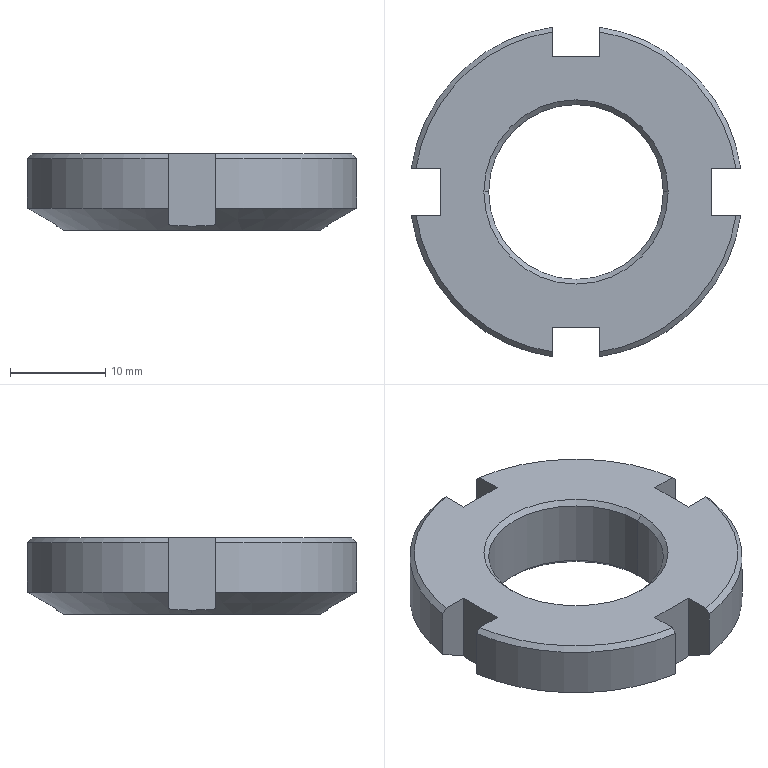Part | STEP file | PN_0042_Default<As Machined> | 1 solid | 30 faces | box 34.641 x 34.641 x 8 mm | volume 4654 mm3 | plane 14 | cone 10 | cylinder 6 | commonest cylinder face diameters 35 x4 18.376 x2
STEP:
#1=CARTESIAN_POINT('',(-9.188,0.,7.5));
#2=VERTEX_POINT('',#1);
#3=CARTESIAN_POINT('',(9.188,0.,7.5));
#4=VERTEX_POINT('',#3);
#5=CARTESIAN_POINT('',(0.,0.,7.5));
#6=DIRECTION('',(0.,0.,1.));
#7=AXIS2_PLACEMENT_3D('',#5,#6,$);
#8=CIRCLE('',#7,9.188);
#9=EDGE_CURVE('',#2,#4,#8,.T.);
#10=ORIENTED_EDGE('',*,*,#9,.F.);
#11=CARTESIAN_POINT('',(-9.688,0.,8.));
#12=VERTEX_POINT('',#11);
#13=CARTESIAN_POINT('',(-353557.985,0.,353556.297));
#14=DIRECTION('',(-0.7071,0.,0.7071));
#15=VECTOR('',#14,1.);
#16=LINE('',#13,#15);
#17=EDGE_CURVE('',#2,#12,#16,.T.);
#18=ORIENTED_EDGE('',*,*,#17,.T.);
#19=CARTESIAN_POINT('',(9.688,0.,8.));
#20=VERTEX_POINT('',#19);
#21=CARTESIAN_POINT('',(0.,0.,8.));
#22=DIRECTION('',(0.,0.,1.));
#23=AXIS2_PLACEMENT_3D('',#21,#22,$);
#24=CIRCLE('',#23,9.688);
#25=EDGE_CURVE('',#20,#12,#24,.F.);
#26=ORIENTED_EDGE('',*,*,#25,.F.);
#27=CARTESIAN_POINT('',(353557.985,0.,353556.297));
#28=DIRECTION('',(0.7071,0.,0.7071));
#29=VECTOR('',#28,1.);
#30=LINE('',#27,#29);
#31=EDGE_CURVE('',#4,#20,#30,.T.);
#32=ORIENTED_EDGE('',*,*,#31,.F.);
#33=EDGE_LOOP('',(#10,#18,#26,#32));
#34=FACE_OUTER_BOUND('',#33,.T.);
#35=CARTESIAN_POINT('',(0.,0.,7.5));
#36=DIRECTION('',(0.,0.,1.));
#37=DIRECTION('',(-1.,0.,0.));
#38=AXIS2_PLACEMENT_3D('',#35,#36,#37);
#39=CONICAL_SURFACE('',#38,9.188,0.7854);
#40=ADVANCED_FACE('',(#34),#39,.F.);
#41=ORIENTED_EDGE('',*,*,#9,.T.);
#42=CARTESIAN_POINT('',(9.188,0.,0.5));
#43=VERTEX_POINT('',#42);
#44=CARTESIAN_POINT('',(9.188,0.,8.));
#45=DIRECTION('',(0.,0.,-1.));
#46=VECTOR('',#45,1.);
#47=LINE('',#44,#46);
#48=EDGE_CURVE('',#4,#43,#47,.T.);
#49=ORIENTED_EDGE('',*,*,#48,.T.);
#50=CARTESIAN_POINT('',(-9.188,0.,0.5));
#51=VERTEX_POINT('',#50);
#52=CARTESIAN_POINT('',(0.,0.,0.5));
#53=DIRECTION('',(0.,0.,-1.));
#54=AXIS2_PLACEMENT_3D('',#52,#53,$);
#55=CIRCLE('',#54,9.188);
#56=EDGE_CURVE('',#43,#51,#55,.T.);
#57=ORIENTED_EDGE('',*,*,#56,.T.);
#58=CARTESIAN_POINT('',(-9.188,0.,8.));
#59=DIRECTION('',(0.,0.,-1.));
#60=VECTOR('',#59,1.);
#61=LINE('',#58,#60);
#62=EDGE_CURVE('',#2,#51,#61,.T.);
#63=ORIENTED_EDGE('',*,*,#62,.F.);
#64=EDGE_LOOP('',(#41,#49,#57,#63));
#65=FACE_OUTER_BOUND('',#64,.T.);
#66=CARTESIAN_POINT('',(0.,0.,8.));
#67=DIRECTION('',(0.,0.,-1.));
#68=DIRECTION('',(1.,0.,0.));
#69=AXIS2_PLACEMENT_3D('',#66,#67,#68);
#70=CYLINDRICAL_SURFACE('',#69,9.188);
#71=ADVANCED_FACE('',(#65),#70,.F.);
#72=ORIENTED_EDGE('',*,*,#17,.F.);
#73=CARTESIAN_POINT('',(0.,0.,7.5));
#74=DIRECTION('',(0.,0.,1.));
#75=AXIS2_PLACEMENT_3D('',#73,#74,$);
#76=CIRCLE('',#75,9.188);
#77=EDGE_CURVE('',#4,#2,#76,.T.);
#78=ORIENTED_EDGE('',*,*,#77,.F.);
#79=ORIENTED_EDGE('',*,*,#31,.T.);
#80=CARTESIAN_POINT('',(0.,0.,8.));
#81=DIRECTION('',(0.,0.,1.));
#82=AXIS2_PLACEMENT_3D('',#80,#81,$);
#83=CIRCLE('',#82,9.688);
#84=EDGE_CURVE('',#12,#20,#83,.F.);
#85=ORIENTED_EDGE('',*,*,#84,.F.);
#86=EDGE_LOOP('',(#72,#78,#79,#85));
#87=FACE_OUTER_BOUND('',#86,.T.);
#88=CARTESIAN_POINT('',(0.,0.,7.5));
#89=DIRECTION('',(0.,0.,1.));
#90=DIRECTION('',(1.,0.,0.));
#91=AXIS2_PLACEMENT_3D('',#88,#89,#90);
#92=CONICAL_SURFACE('',#91,9.188,0.7854);
#93=ADVANCED_FACE('',(#87),#92,.F.);
#94=CARTESIAN_POINT('',(16.815,2.5,8.));
#95=VERTEX_POINT('',#94);
#96=CARTESIAN_POINT('',(14.221,2.5,8.));
#97=VERTEX_POINT('',#96);
#98=CARTESIAN_POINT('',(15.518,2.5,8.));
#99=DIRECTION('',(-1.,0.,0.));
#100=VECTOR('',#99,1.);
#101=LINE('',#98,#100);
#102=EDGE_CURVE('',#95,#97,#101,.T.);
#103=ORIENTED_EDGE('',*,*,#102,.F.);
#104=CARTESIAN_POINT('',(2.5,16.815,8.));
#105=VERTEX_POINT('',#104);
#106=CARTESIAN_POINT('',(-0.000000003,-0.000000003,8.));
#107=DIRECTION('',(0.,0.,1.));
#108=AXIS2_PLACEMENT_3D('',#106,#107,$);
#109=CIRCLE('',#108,17.);
#110=EDGE_CURVE('',#95,#105,#109,.T.);
#111=ORIENTED_EDGE('',*,*,#110,.T.);
#112=CARTESIAN_POINT('',(2.5,14.221,8.));
#113=VERTEX_POINT('',#112);
#114=CARTESIAN_POINT('',(2.5,15.518,8.));
#115=DIRECTION('',(0.,1.,0.));
#116=VECTOR('',#115,1.);
#117=LINE('',#114,#116);
#118=EDGE_CURVE('',#113,#105,#117,.T.);
#119=ORIENTED_EDGE('',*,*,#118,.F.);
#120=CARTESIAN_POINT('',(-2.5,14.221,8.));
#121=VERTEX_POINT('',#120);
#122=CARTESIAN_POINT('',(0.,14.221,8.));
#123=DIRECTION('',(1.,0.,0.));
#124=VECTOR('',#123,1.);
#125=LINE('',#122,#124);
#126=EDGE_CURVE('',#121,#113,#125,.T.);
#127=ORIENTED_EDGE('',*,*,#126,.F.);
#128=CARTESIAN_POINT('',(-2.5,16.815,8.));
#129=VERTEX_POINT('',#128);
#130=CARTESIAN_POINT('',(-2.5,15.518,8.));
#131=DIRECTION('',(0.,-1.,0.));
#132=VECTOR('',#131,1.);
#133=LINE('',#130,#132);
#134=EDGE_CURVE('',#129,#121,#133,.T.);
#135=ORIENTED_EDGE('',*,*,#134,.F.);
#136=CARTESIAN_POINT('',(-16.815,2.5,8.));
#137=VERTEX_POINT('',#136);
#138=CARTESIAN_POINT('',(0.000000003,-0.000000003,8.));
#139=DIRECTION('',(0.,0.,1.));
#140=AXIS2_PLACEMENT_3D('',#138,#139,$);
#141=CIRCLE('',#140,17.);
#142=EDGE_CURVE('',#129,#137,#141,.T.);
#143=ORIENTED_EDGE('',*,*,#142,.T.);
#144=CARTESIAN_POINT('',(-14.221,2.5,8.));
#145=VERTEX_POINT('',#144);
#146=CARTESIAN_POINT('',(-15.518,2.5,8.));
#147=DIRECTION('',(-1.,0.,0.));
#148=VECTOR('',#147,1.);
#149=LINE('',#146,#148);
#150=EDGE_CURVE('',#145,#137,#149,.T.);
#151=ORIENTED_EDGE('',*,*,#150,.F.);
#152=CARTESIAN_POINT('',(-14.221,-2.5,8.));
#153=VERTEX_POINT('',#152);
#154=CARTESIAN_POINT('',(-14.221,0.,8.));
#155=DIRECTION('',(0.,1.,0.));
#156=VECTOR('',#155,1.);
#157=LINE('',#154,#156);
#158=EDGE_CURVE('',#153,#145,#157,.T.);
#159=ORIENTED_EDGE('',*,*,#158,.F.);
#160=CARTESIAN_POINT('',(-16.815,-2.5,8.));
#161=VERTEX_POINT('',#160);
#162=CARTESIAN_POINT('',(-15.518,-2.5,8.));
#163=DIRECTION('',(1.,0.,0.));
#164=VECTOR('',#163,1.);
#165=LINE('',#162,#164);
#166=EDGE_CURVE('',#161,#153,#165,.T.);
#167=ORIENTED_EDGE('',*,*,#166,.F.);
#168=CARTESIAN_POINT('',(-2.5,-16.815,8.));
#169=VERTEX_POINT('',#168);
#170=CARTESIAN_POINT('',(0.000000003,0.000000003,8.));
#171=DIRECTION('',(0.,0.,1.));
#172=AXIS2_PLACEMENT_3D('',#170,#171,$);
#173=CIRCLE('',#172,17.);
#174=EDGE_CURVE('',#161,#169,#173,.T.);
#175=ORIENTED_EDGE('',*,*,#174,.T.);
#176=CARTESIAN_POINT('',(-2.5,-14.221,8.));
#177=VERTEX_POINT('',#176);
#178=CARTESIAN_POINT('',(-2.5,-15.518,8.));
#179=DIRECTION('',(0.,-1.,0.));
#180=VECTOR('',#179,1.);
#181=LINE('',#178,#180);
#182=EDGE_CURVE('',#177,#169,#181,.T.);
#183=ORIENTED_EDGE('',*,*,#182,.F.);
#184=CARTESIAN_POINT('',(2.5,-14.221,8.));
#185=VERTEX_POINT('',#184);
#186=CARTESIAN_POINT('',(0.,-14.221,8.));
#187=DIRECTION('',(-1.,0.,0.));
#188=VECTOR('',#187,1.);
#189=LINE('',#186,#188);
#190=EDGE_CURVE('',#185,#177,#189,.T.);
#191=ORIENTED_EDGE('',*,*,#190,.F.);
#192=CARTESIAN_POINT('',(2.5,-16.815,8.));
#193=VERTEX_POINT('',#192);
#194=CARTESIAN_POINT('',(2.5,-15.518,8.));
#195=DIRECTION('',(0.,1.,0.));
#196=VECTOR('',#195,1.);
#197=LINE('',#194,#196);
#198=EDGE_CURVE('',#193,#185,#197,.T.);
#199=ORIENTED_EDGE('',*,*,#198,.F.);
#200=CARTESIAN_POINT('',(16.815,-2.5,8.));
#201=VERTEX_POINT('',#200);
#202=CARTESIAN_POINT('',(-0.000000003,0.000000003,8.));
#203=DIRECTION('',(0.,0.,1.));
#204=AXIS2_PLACEMENT_3D('',#202,#203,$);
#205=CIRCLE('',#204,17.);
#206=EDGE_CURVE('',#193,#201,#205,.T.);
#207=ORIENTED_EDGE('',*,*,#206,.T.);
#208=CARTESIAN_POINT('',(14.221,-2.5,8.));
#209=VERTEX_POINT('',#208);
#210=CARTESIAN_POINT('',(15.518,-2.5,8.));
#211=DIRECTION('',(1.,0.,0.));
#212=VECTOR('',#211,1.);
#213=LINE('',#210,#212);
#214=EDGE_CURVE('',#209,#201,#213,.T.);
#215=ORIENTED_EDGE('',*,*,#214,.F.);
#216=CARTESIAN_POINT('',(14.221,0.,8.));
#217=DIRECTION('',(0.,-1.,0.));
#218=VECTOR('',#217,1.);
#219=LINE('',#216,#218);
#220=EDGE_CURVE('',#97,#209,#219,.T.);
#221=ORIENTED_EDGE('',*,*,#220,.F.);
#222=EDGE_LOOP('',(#103,#111,#119,#127,#135,#143,#151,#159,#167,#175,#183,#191,#199,#207,#215,#221));
#223=FACE_OUTER_BOUND('',#222,.T.);
#224=ORIENTED_EDGE('',*,*,#25,.T.);
#225=ORIENTED_EDGE('',*,*,#84,.T.);
#226=EDGE_LOOP('',(#224,#225));
#227=FACE_BOUND('',#226,.T.);
#228=CARTESIAN_POINT('',(0.,0.,8.));
#229=DIRECTION('',(0.,0.,1.));
#230=DIRECTION('',(1.,0.,0.));
#231=AXIS2_PLACEMENT_3D('',#228,#229,#230);
#232=PLANE('',#231);
#233=ADVANCED_FACE('',(#223,#227),#232,.T.);
#234=ORIENTED_EDGE('',*,*,#48,.F.);
#235=ORIENTED_EDGE('',*,*,#77,.T.);
#236=ORIENTED_EDGE('',*,*,#62,.T.);
#237=CARTESIAN_POINT('',(0.,0.,0.5));
#238=DIRECTION('',(0.,0.,-1.));
#239=AXIS2_PLACEMENT_3D('',#237,#238,$);
#240=CIRCLE('',#239,9.188);
#241=EDGE_CURVE('',#51,#43,#240,.T.);
#242=ORIENTED_EDGE('',*,*,#241,.T.);
#243=EDGE_LOOP('',(#234,#235,#236,#242));
#244=FACE_OUTER_BOUND('',#243,.T.);
#245=CARTESIAN_POINT('',(0.,0.,8.));
#246=DIRECTION('',(0.,0.,-1.));
#247=DIRECTION('',(-1.,0.,0.));
#248=AXIS2_PLACEMENT_3D('',#245,#246,#247);
#249=CYLINDRICAL_SURFACE('',#248,9.188);
#250=ADVANCED_FACE('',(#244),#249,.F.);
#251=ORIENTED_EDGE('',*,*,#56,.F.);
#252=CARTESIAN_POINT('',(9.688,0.,0.));
#253=VERTEX_POINT('',#252);
#254=CARTESIAN_POINT('',(353558.235,0.,-353548.547));
#255=DIRECTION('',(0.7071,0.,-0.7071));
#256=VECTOR('',#255,1.);
#257=LINE('',#254,#256);
#258=EDGE_CURVE('',#43,#253,#257,.T.);
#259=ORIENTED_EDGE('',*,*,#258,.T.);
#260=CARTESIAN_POINT('',(-9.688,0.,0.));
#261=VERTEX_POINT('',#260);
#262=CARTESIAN_POINT('',(0.,0.,0.));
#263=DIRECTION('',(0.,0.,-1.));
#264=AXIS2_PLACEMENT_3D('',#262,#263,$);
#265=CIRCLE('',#264,9.688);
#266=EDGE_CURVE('',#261,#253,#265,.F.);
#267=ORIENTED_EDGE('',*,*,#266,.F.);
#268=CARTESIAN_POINT('',(-353558.235,0.,-353548.547));
#269=DIRECTION('',(-0.7071,0.,-0.7071));
#270=VECTOR('',#269,1.);
#271=LINE('',#268,#270);
#272=EDGE_CURVE('',#51,#261,#271,.T.);
#273=ORIENTED_EDGE('',*,*,#272,.F.);
#274=EDGE_LOOP('',(#251,#259,#267,#273));
#275=FACE_OUTER_BOUND('',#274,.T.);
#276=CARTESIAN_POINT('',(0.,0.,0.));
#277=DIRECTION('',(0.,0.,-1.));
#278=DIRECTION('',(1.,0.,0.));
#279=AXIS2_PLACEMENT_3D('',#276,#277,#278);
#280=CONICAL_SURFACE('',#279,9.688,0.7854);
#281=ADVANCED_FACE('',(#275),#280,.F.);
#282=CARTESIAN_POINT('',(17.321,2.5,7.5));
#283=VERTEX_POINT('',#282);
#284=CARTESIAN_POINT('',(17.321,2.5,7.5));
#285=CARTESIAN_POINT('',(17.219,2.5,7.6));
#286=CARTESIAN_POINT('',(17.118,2.5,7.7));
#287=CARTESIAN_POINT('',(17.017,2.5,7.8));
#288=CARTESIAN_POINT('',(16.916,2.5,7.9));
#289=CARTESIAN_POINT('',(16.815,2.5,8.));
#290=B_SPLINE_CURVE_WITH_KNOTS('',5,(#284,#285,#286,#287,#288,#289),.UNSPECIFIED.,.F.,.U.,(6,6),(0.,1.005),.UNSPECIFIED.);
#291=EDGE_CURVE('',#283,#95,#290,.T.);
#292=ORIENTED_EDGE('',*,*,#291,.T.);
#293=ORIENTED_EDGE('',*,*,#102,.T.);
#294=CARTESIAN_POINT('',(14.221,2.5,0.5419));
#295=VERTEX_POINT('',#294);
#296=CARTESIAN_POINT('',(14.221,2.5,4.271));
#297=DIRECTION('',(0.,0.,1.));
#298=VECTOR('',#297,1.);
#299=LINE('',#296,#298);
#300=EDGE_CURVE('',#295,#97,#299,.T.);
#301=ORIENTED_EDGE('',*,*,#300,.F.);
#302=CARTESIAN_POINT('',(17.321,2.5,2.309));
#303=VERTEX_POINT('',#302);
#304=CARTESIAN_POINT('',(14.221,2.5,0.5419));
#305=CARTESIAN_POINT('',(14.841,2.5,0.8947));
#306=CARTESIAN_POINT('',(15.461,2.5,1.248));
#307=CARTESIAN_POINT('',(16.081,2.5,1.601));
#308=CARTESIAN_POINT('',(16.701,2.5,1.955));
#309=CARTESIAN_POINT('',(17.321,2.5,2.309));
#310=B_SPLINE_CURVE_WITH_KNOTS('',5,(#304,#305,#306,#307,#308,#309),.UNSPECIFIED.,.F.,.U.,(6,6),(0.,5.047),.UNSPECIFIED.);
#311=EDGE_CURVE('',#295,#303,#310,.T.);
#312=ORIENTED_EDGE('',*,*,#311,.T.);
#313=CARTESIAN_POINT('',(17.321,2.5,4.905));
#314=DIRECTION('',(0.,0.,1.));
#315=VECTOR('',#314,1.);
#316=LINE('',#313,#315);
#317=EDGE_CURVE('',#303,#283,#316,.T.);
#318=ORIENTED_EDGE('',*,*,#317,.T.);
#319=EDGE_LOOP('',(#292,#293,#301,#312,#318));
#320=FACE_OUTER_BOUND('',#319,.T.);
#321=CARTESIAN_POINT('',(14.221,2.5,0.));
#322=DIRECTION('',(0.,1.,0.));
#323=DIRECTION('',(-1.,0.,0.));
#324=AXIS2_PLACEMENT_3D('',#321,#322,#323);
#325=PLANE('',#324);
#326=ADVANCED_FACE('',(#320),#325,.F.);
#327=ORIENTED_EDGE('',*,*,#291,.F.);
#328=CARTESIAN_POINT('',(2.5,17.321,7.5));
#329=VERTEX_POINT('',#328);
#330=CARTESIAN_POINT('',(0.,0.,7.5));
#331=DIRECTION('',(0.,0.,-1.));
#332=AXIS2_PLACEMENT_3D('',#330,#331,$);
#333=CIRCLE('',#332,17.5);
#334=EDGE_CURVE('',#329,#283,#333,.T.);
#335=ORIENTED_EDGE('',*,*,#334,.F.);
#336=CARTESIAN_POINT('',(2.5,16.815,8.));
#337=CARTESIAN_POINT('',(2.5,16.983,7.834));
#338=CARTESIAN_POINT('',(2.5,17.151,7.667));
#339=CARTESIAN_POINT('',(2.5,17.321,7.5));
#340=B_SPLINE_CURVE_WITH_KNOTS('',3,(#336,#337,#338,#339),.UNSPECIFIED.,.F.,.U.,(4,4),(0.,1.089),.UNSPECIFIED.);
#341=EDGE_CURVE('',#105,#329,#340,.T.);
#342=ORIENTED_EDGE('',*,*,#341,.F.);
#343=ORIENTED_EDGE('',*,*,#110,.F.);
#344=EDGE_LOOP('',(#327,#335,#342,#343));
#345=FACE_OUTER_BOUND('',#344,.T.);
#346=CARTESIAN_POINT('',(0.,0.,8.));
#347=DIRECTION('',(0.,0.,-1.));
#348=DIRECTION('',(-1.,0.,0.));
#349=AXIS2_PLACEMENT_3D('',#346,#347,#348);
#350=CONICAL_SURFACE('',#349,17.,0.7854);
#351=ADVANCED_FACE('',(#345),#350,.T.);
#352=ORIENTED_EDGE('',*,*,#341,.T.);
#353=CARTESIAN_POINT('',(2.5,17.321,2.309));
#354=VERTEX_POINT('',#353);
#355=CARTESIAN_POINT('',(2.5,17.321,4.905));
#356=DIRECTION('',(0.,0.,1.));
#357=VECTOR('',#356,1.);
#358=LINE('',#355,#357);
#359=EDGE_CURVE('',#354,#329,#358,.T.);
#360=ORIENTED_EDGE('',*,*,#359,.F.);
#361=CARTESIAN_POINT('',(2.5,14.221,0.5419));
#362=VERTEX_POINT('',#361);
#363=CARTESIAN_POINT('',(2.5,17.321,2.309));
#364=CARTESIAN_POINT('',(2.5,16.701,1.955));
#365=CARTESIAN_POINT('',(2.5,16.081,1.601));
#366=CARTESIAN_POINT('',(2.5,15.461,1.248));
#367=CARTESIAN_POINT('',(2.5,14.841,0.8947));
#368=CARTESIAN_POINT('',(2.5,14.221,0.5419));
#369=B_SPLINE_CURVE_WITH_KNOTS('',5,(#363,#364,#365,#366,#367,#368),.UNSPECIFIED.,.F.,.U.,(6,6),(0.,5.047),.UNSPECIFIED.);
#370=EDGE_CURVE('',#354,#362,#369,.T.);
#371=ORIENTED_EDGE('',*,*,#370,.T.);
#372=CARTESIAN_POINT('',(2.5,14.221,4.271));
#373=DIRECTION('',(0.,0.,1.));
#374=VECTOR('',#373,1.);
#375=LINE('',#372,#374);
#376=EDGE_CURVE('',#362,#113,#375,.T.);
#377=ORIENTED_EDGE('',*,*,#376,.T.);
#378=ORIENTED_EDGE('',*,*,#118,.T.);
#379=EDGE_LOOP('',(#352,#360,#371,#377,#378));
#380=FACE_OUTER_BOUND('',#379,.T.);
#381=CARTESIAN_POINT('',(2.5,14.221,0.));
#382=DIRECTION('',(1.,0.,0.));
#383=DIRECTION('',(0.,1.,0.));
#384=AXIS2_PLACEMENT_3D('',#381,#382,#383);
#385=PLANE('',#384);
#386=ADVANCED_FACE('',(#380),#385,.F.);
#387=CARTESIAN_POINT('',(-2.5,14.221,0.5419));
#388=VERTEX_POINT('',#387);
#389=CARTESIAN_POINT('',(2.5,14.221,0.5419));
#390=CARTESIAN_POINT('',(1.904,14.221,0.4823));
#391=CARTESIAN_POINT('',(1.307,14.221,0.44));
#392=CARTESIAN_POINT('',(0.7073,14.221,0.4152));
#393=CARTESIAN_POINT('',(-0.2936,14.221,0.4047));
#394=CARTESIAN_POINT('',(-1.296,14.221,0.4451));
#395=CARTESIAN_POINT('',(-1.697,14.221,0.4695));
#396=CARTESIAN_POINT('',(-2.099,14.221,0.5018));
#397=CARTESIAN_POINT('',(-2.5,14.221,0.5419));
#398=B_SPLINE_CURVE_WITH_KNOTS('',5,(#389,#390,#391,#392,#393,#394,#395,#396,#397),.UNSPECIFIED.,.F.,.U.,(6,3,6),(0.,4.243,7.085),.UNSPECIFIED.);
#399=EDGE_CURVE('',#362,#388,#398,.T.);
#400=ORIENTED_EDGE('',*,*,#399,.T.);
#401=CARTESIAN_POINT('',(-2.5,14.221,4.271));
#402=DIRECTION('',(0.,0.,1.));
#403=VECTOR('',#402,1.);
#404=LINE('',#401,#403);
#405=EDGE_CURVE('',#388,#121,#404,.T.);
#406=ORIENTED_EDGE('',*,*,#405,.T.);
#407=ORIENTED_EDGE('',*,*,#126,.T.);
#408=ORIENTED_EDGE('',*,*,#376,.F.);
#409=EDGE_LOOP('',(#400,#406,#407,#408));
#410=FACE_OUTER_BOUND('',#409,.T.);
#411=CARTESIAN_POINT('',(2.5,14.221,0.));
#412=DIRECTION('',(0.,-1.,0.));
#413=DIRECTION('',(1.,0.,0.));
#414=AXIS2_PLACEMENT_3D('',#411,#412,#413);
#415=PLANE('',#414);
#416=ADVANCED_FACE('',(#410),#415,.F.);
#417=CARTESIAN_POINT('',(-2.5,17.321,7.5));
#418=VERTEX_POINT('',#417);
#419=CARTESIAN_POINT('',(-2.5,17.321,7.5));
#420=CARTESIAN_POINT('',(-2.5,17.219,7.6));
#421=CARTESIAN_POINT('',(-2.5,17.118,7.7));
#422=CARTESIAN_POINT('',(-2.5,17.017,7.8));
#423=CARTESIAN_POINT('',(-2.5,16.916,7.9));
#424=CARTESIAN_POINT('',(-2.5,16.815,8.));
#425=B_SPLINE_CURVE_WITH_KNOTS('',5,(#419,#420,#421,#422,#423,#424),.UNSPECIFIED.,.F.,.U.,(6,6),(0.,1.005),.UNSPECIFIED.);
#426=EDGE_CURVE('',#418,#129,#425,.T.);
#427=ORIENTED_EDGE('',*,*,#426,.T.);
#428=ORIENTED_EDGE('',*,*,#134,.T.);
#429=ORIENTED_EDGE('',*,*,#405,.F.);
#430=CARTESIAN_POINT('',(-2.5,17.321,2.309));
#431=VERTEX_POINT('',#430);
#432=CARTESIAN_POINT('',(-2.5,14.221,0.5419));
#433=CARTESIAN_POINT('',(-2.5,14.841,0.8947));
#434=CARTESIAN_POINT('',(-2.5,15.461,1.248));
#435=CARTESIAN_POINT('',(-2.5,16.081,1.601));
#436=CARTESIAN_POINT('',(-2.5,16.701,1.955));
#437=CARTESIAN_POINT('',(-2.5,17.321,2.309));
#438=B_SPLINE_CURVE_WITH_KNOTS('',5,(#432,#433,#434,#435,#436,#437),.UNSPECIFIED.,.F.,.U.,(6,6),(0.,5.047),.UNSPECIFIED.);
#439=EDGE_CURVE('',#388,#431,#438,.T.);
#440=ORIENTED_EDGE('',*,*,#439,.T.);
#441=CARTESIAN_POINT('',(-2.5,17.321,4.905));
#442=DIRECTION('',(0.,0.,1.));
#443=VECTOR('',#442,1.);
#444=LINE('',#441,#443);
#445=EDGE_CURVE('',#431,#418,#444,.T.);
#446=ORIENTED_EDGE('',*,*,#445,.T.);
#447=EDGE_LOOP('',(#427,#428,#429,#440,#446));
#448=FACE_OUTER_BOUND('',#447,.T.);
#449=CARTESIAN_POINT('',(-2.5,14.221,0.));
#450=DIRECTION('',(-1.,0.,0.));
#451=DIRECTION('',(0.,-1.,0.));
#452=AXIS2_PLACEMENT_3D('',#449,#450,#451);
#453=PLANE('',#452);
#454=ADVANCED_FACE('',(#448),#453,.F.);
#455=ORIENTED_EDGE('',*,*,#426,.F.);
#456=CARTESIAN_POINT('',(-17.321,2.5,7.5));
#457=VERTEX_POINT('',#456);
#458=CARTESIAN_POINT('',(0.,0.,7.5));
#459=DIRECTION('',(0.,0.,-1.));
#460=AXIS2_PLACEMENT_3D('',#458,#459,$);
#461=CIRCLE('',#460,17.5);
#462=EDGE_CURVE('',#457,#418,#461,.T.);
#463=ORIENTED_EDGE('',*,*,#462,.F.);
#464=CARTESIAN_POINT('',(-16.815,2.5,8.));
#465=CARTESIAN_POINT('',(-16.983,2.5,7.834));
#466=CARTESIAN_POINT('',(-17.151,2.5,7.667));
#467=CARTESIAN_POINT('',(-17.321,2.5,7.5));
#468=B_SPLINE_CURVE_WITH_KNOTS('',3,(#464,#465,#466,#467),.UNSPECIFIED.,.F.,.U.,(4,4),(0.,1.089),.UNSPECIFIED.);
#469=EDGE_CURVE('',#137,#457,#468,.T.);
#470=ORIENTED_EDGE('',*,*,#469,.F.);
#471=ORIENTED_EDGE('',*,*,#142,.F.);
#472=EDGE_LOOP('',(#455,#463,#470,#471));
#473=FACE_OUTER_BOUND('',#472,.T.);
#474=CARTESIAN_POINT('',(0.,0.,8.));
#475=DIRECTION('',(0.,0.,-1.));
#476=DIRECTION('',(-1.,0.,0.));
#477=AXIS2_PLACEMENT_3D('',#474,#475,#476);
#478=CONICAL_SURFACE('',#477,17.,0.7854);
#479=ADVANCED_FACE('',(#473),#478,.T.);
#480=ORIENTED_EDGE('',*,*,#469,.T.);
#481=CARTESIAN_POINT('',(-17.321,2.5,2.309));
#482=VERTEX_POINT('',#481);
#483=CARTESIAN_POINT('',(-17.321,2.5,4.905));
#484=DIRECTION('',(0.,0.,1.));
#485=VECTOR('',#484,1.);
#486=LINE('',#483,#485);
#487=EDGE_CURVE('',#482,#457,#486,.T.);
#488=ORIENTED_EDGE('',*,*,#487,.F.);
#489=CARTESIAN_POINT('',(-14.221,2.5,0.5419));
#490=VERTEX_POINT('',#489);
#491=CARTESIAN_POINT('',(-17.321,2.5,2.309));
#492=CARTESIAN_POINT('',(-16.701,2.5,1.955));
#493=CARTESIAN_POINT('',(-16.081,2.5,1.601));
#494=CARTESIAN_POINT('',(-15.461,2.5,1.248));
#495=CARTESIAN_POINT('',(-14.841,2.5,0.8947));
#496=CARTESIAN_POINT('',(-14.221,2.5,0.5419));
#497=B_SPLINE_CURVE_WITH_KNOTS('',5,(#491,#492,#493,#494,#495,#496),.UNSPECIFIED.,.F.,.U.,(6,6),(0.,5.047),.UNSPECIFIED.);
#498=EDGE_CURVE('',#482,#490,#497,.T.);
#499=ORIENTED_EDGE('',*,*,#498,.T.);
#500=CARTESIAN_POINT('',(-14.221,2.5,4.271));
#501=DIRECTION('',(0.,0.,1.));
#502=VECTOR('',#501,1.);
#503=LINE('',#500,#502);
#504=EDGE_CURVE('',#490,#145,#503,.T.);
#505=ORIENTED_EDGE('',*,*,#504,.T.);
#506=ORIENTED_EDGE('',*,*,#150,.T.);
#507=EDGE_LOOP('',(#480,#488,#499,#505,#506));
#508=FACE_OUTER_BOUND('',#507,.T.);
#509=CARTESIAN_POINT('',(-14.221,2.5,0.));
#510=DIRECTION('',(0.,1.,0.));
#511=DIRECTION('',(-1.,0.,0.));
#512=AXIS2_PLACEMENT_3D('',#509,#510,#511);
#513=PLANE('',#512);
#514=ADVANCED_FACE('',(#508),#513,.F.);
#515=CARTESIAN_POINT('',(-14.221,0.,0.416));
#516=VERTEX_POINT('',#515);
#517=CARTESIAN_POINT('',(-14.221,2.5,0.5419));
#518=CARTESIAN_POINT('',(-14.221,2.002,0.4921));
#519=CARTESIAN_POINT('',(-14.221,1.503,0.4543));
#520=CARTESIAN_POINT('',(-14.221,1.002,0.4288));
#521=CARTESIAN_POINT('',(-14.221,0.5013,0.416));
#522=CARTESIAN_POINT('',(-14.221,0.,0.416));
#523=B_SPLINE_CURVE_WITH_KNOTS('',5,(#517,#518,#519,#520,#521,#522),.UNSPECIFIED.,.F.,.U.,(6,6),(0.,3.541),.UNSPECIFIED.);
#524=EDGE_CURVE('',#490,#516,#523,.T.);
#525=ORIENTED_EDGE('',*,*,#524,.T.);
#526=CARTESIAN_POINT('',(-14.221,-2.5,0.5419));
#527=VERTEX_POINT('',#526);
#528=CARTESIAN_POINT('',(-14.221,0.,0.416));
#529=CARTESIAN_POINT('',(-14.221,-0.2993,0.416));
#530=CARTESIAN_POINT('',(-14.221,-0.5986,0.4205));
#531=CARTESIAN_POINT('',(-14.221,-0.8998,0.4297));
#532=CARTESIAN_POINT('',(-14.221,-1.4,0.4525));
#533=CARTESIAN_POINT('',(-14.221,-1.9,0.4878));
#534=CARTESIAN_POINT('',(-14.221,-2.1,0.5039));
#535=CARTESIAN_POINT('',(-14.221,-2.3,0.5219));
#536=CARTESIAN_POINT('',(-14.221,-2.5,0.5419));
#537=B_SPLINE_CURVE_WITH_KNOTS('',5,(#528,#529,#530,#531,#532,#533,#534,#535,#536),.UNSPECIFIED.,.F.,.U.,(6,3,6),(0.,2.121,3.539),.UNSPECIFIED.);
#538=EDGE_CURVE('',#516,#527,#537,.T.);
#539=ORIENTED_EDGE('',*,*,#538,.T.);
#540=CARTESIAN_POINT('',(-14.221,-2.5,4.271));
#541=DIRECTION('',(0.,0.,1.));
#542=VECTOR('',#541,1.);
#543=LINE('',#540,#542);
#544=EDGE_CURVE('',#527,#153,#543,.T.);
#545=ORIENTED_EDGE('',*,*,#544,.T.);
#546=ORIENTED_EDGE('',*,*,#158,.T.);
#547=ORIENTED_EDGE('',*,*,#504,.F.);
#548=EDGE_LOOP('',(#525,#539,#545,#546,#547));
#549=FACE_OUTER_BOUND('',#548,.T.);
#550=CARTESIAN_POINT('',(-14.221,2.5,0.));
#551=DIRECTION('',(1.,0.,0.));
#552=DIRECTION('',(0.,1.,0.));
#553=AXIS2_PLACEMENT_3D('',#550,#551,#552);
#554=PLANE('',#553);
#555=ADVANCED_FACE('',(#549),#554,.F.);
#556=CARTESIAN_POINT('',(-17.321,-2.5,7.5));
#557=VERTEX_POINT('',#556);
#558=CARTESIAN_POINT('',(-17.321,-2.5,7.5));
#559=CARTESIAN_POINT('',(-17.219,-2.5,7.6));
#560=CARTESIAN_POINT('',(-17.118,-2.5,7.7));
#561=CARTESIAN_POINT('',(-17.017,-2.5,7.8));
#562=CARTESIAN_POINT('',(-16.916,-2.5,7.9));
#563=CARTESIAN_POINT('',(-16.815,-2.5,8.));
#564=B_SPLINE_CURVE_WITH_KNOTS('',5,(#558,#559,#560,#561,#562,#563),.UNSPECIFIED.,.F.,.U.,(6,6),(0.,1.005),.UNSPECIFIED.);
#565=EDGE_CURVE('',#557,#161,#564,.T.);
#566=ORIENTED_EDGE('',*,*,#565,.T.);
#567=ORIENTED_EDGE('',*,*,#166,.T.);
#568=ORIENTED_EDGE('',*,*,#544,.F.);
#569=CARTESIAN_POINT('',(-17.321,-2.5,2.309));
#570=VERTEX_POINT('',#569);
#571=CARTESIAN_POINT('',(-14.221,-2.5,0.5419));
#572=CARTESIAN_POINT('',(-14.841,-2.5,0.8947));
#573=CARTESIAN_POINT('',(-15.461,-2.5,1.248));
#574=CARTESIAN_POINT('',(-16.081,-2.5,1.601));
#575=CARTESIAN_POINT('',(-16.701,-2.5,1.955));
#576=CARTESIAN_POINT('',(-17.321,-2.5,2.309));
#577=B_SPLINE_CURVE_WITH_KNOTS('',5,(#571,#572,#573,#574,#575,#576),.UNSPECIFIED.,.F.,.U.,(6,6),(0.,5.047),.UNSPECIFIED.);
#578=EDGE_CURVE('',#527,#570,#577,.T.);
#579=ORIENTED_EDGE('',*,*,#578,.T.);
#580=CARTESIAN_POINT('',(-17.321,-2.5,4.905));
#581=DIRECTION('',(0.,0.,1.));
#582=VECTOR('',#581,1.);
#583=LINE('',#580,#582);
#584=EDGE_CURVE('',#570,#557,#583,.T.);
#585=ORIENTED_EDGE('',*,*,#584,.T.);
#586=EDGE_LOOP('',(#566,#567,#568,#579,#585));
#587=FACE_OUTER_BOUND('',#586,.T.);
#588=CARTESIAN_POINT('',(-14.221,-2.5,0.));
#589=DIRECTION('',(0.,-1.,0.));
#590=DIRECTION('',(1.,0.,0.));
#591=AXIS2_PLACEMENT_3D('',#588,#589,#590);
#592=PLANE('',#591);
#593=ADVANCED_FACE('',(#587),#592,.F.);
#594=ORIENTED_EDGE('',*,*,#565,.F.);
#595=CARTESIAN_POINT('',(-2.5,-17.321,7.5));
#596=VERTEX_POINT('',#595);
#597=CARTESIAN_POINT('',(0.,0.,7.5));
#598=DIRECTION('',(0.,0.,-1.));
#599=AXIS2_PLACEMENT_3D('',#597,#598,$);
#600=CIRCLE('',#599,17.5);
#601=EDGE_CURVE('',#596,#557,#600,.T.);
#602=ORIENTED_EDGE('',*,*,#601,.F.);
#603=CARTESIAN_POINT('',(-2.5,-16.815,8.));
#604=CARTESIAN_POINT('',(-2.5,-16.983,7.834));
#605=CARTESIAN_POINT('',(-2.5,-17.151,7.667));
#606=CARTESIAN_POINT('',(-2.5,-17.321,7.5));
#607=B_SPLINE_CURVE_WITH_KNOTS('',3,(#603,#604,#605,#606),.UNSPECIFIED.,.F.,.U.,(4,4),(0.,1.089),.UNSPECIFIED.);
#608=EDGE_CURVE('',#169,#596,#607,.T.);
#609=ORIENTED_EDGE('',*,*,#608,.F.);
#610=ORIENTED_EDGE('',*,*,#174,.F.);
#611=EDGE_LOOP('',(#594,#602,#609,#610));
#612=FACE_OUTER_BOUND('',#611,.T.);
#613=CARTESIAN_POINT('',(0.,0.,8.));
#614=DIRECTION('',(0.,0.,-1.));
#615=DIRECTION('',(1.,0.,0.));
#616=AXIS2_PLACEMENT_3D('',#613,#614,#615);
#617=CONICAL_SURFACE('',#616,17.,0.7854);
#618=ADVANCED_FACE('',(#612),#617,.T.);
#619=ORIENTED_EDGE('',*,*,#608,.T.);
#620=CARTESIAN_POINT('',(-2.5,-17.321,2.309));
#621=VERTEX_POINT('',#620);
#622=CARTESIAN_POINT('',(-2.5,-17.321,4.905));
#623=DIRECTION('',(0.,0.,1.));
#624=VECTOR('',#623,1.);
#625=LINE('',#622,#624);
#626=EDGE_CURVE('',#621,#596,#625,.T.);
#627=ORIENTED_EDGE('',*,*,#626,.F.);
#628=CARTESIAN_POINT('',(-2.5,-14.221,0.5419));
#629=VERTEX_POINT('',#628);
#630=CARTESIAN_POINT('',(-2.5,-17.321,2.309));
#631=CARTESIAN_POINT('',(-2.5,-16.701,1.955));
#632=CARTESIAN_POINT('',(-2.5,-16.081,1.601));
#633=CARTESIAN_POINT('',(-2.5,-15.461,1.248));
#634=CARTESIAN_POINT('',(-2.5,-14.841,0.8947));
#635=CARTESIAN_POINT('',(-2.5,-14.221,0.5419));
#636=B_SPLINE_CURVE_WITH_KNOTS('',5,(#630,#631,#632,#633,#634,#635),.UNSPECIFIED.,.F.,.U.,(6,6),(0.,5.047),.UNSPECIFIED.);
#637=EDGE_CURVE('',#621,#629,#636,.T.);
#638=ORIENTED_EDGE('',*,*,#637,.T.);
#639=CARTESIAN_POINT('',(-2.5,-14.221,4.271));
#640=DIRECTION('',(0.,0.,1.));
#641=VECTOR('',#640,1.);
#642=LINE('',#639,#641);
#643=EDGE_CURVE('',#629,#177,#642,.T.);
#644=ORIENTED_EDGE('',*,*,#643,.T.);
#645=ORIENTED_EDGE('',*,*,#182,.T.);
#646=EDGE_LOOP('',(#619,#627,#638,#644,#645));
#647=FACE_OUTER_BOUND('',#646,.T.);
#648=CARTESIAN_POINT('',(-2.5,-14.221,0.));
#649=DIRECTION('',(-1.,0.,0.));
#650=DIRECTION('',(0.,0.,1.));
#651=AXIS2_PLACEMENT_3D('',#648,#649,#650);
#652=PLANE('',#651);
#653=ADVANCED_FACE('',(#647),#652,.F.);
#654=CARTESIAN_POINT('',(2.5,-14.221,0.5419));
#655=VERTEX_POINT('',#654);
#656=CARTESIAN_POINT('',(-2.5,-14.221,0.5419));
#657=CARTESIAN_POINT('',(-2.099,-14.221,0.5018));
#658=CARTESIAN_POINT('',(-1.697,-14.221,0.4695));
#659=CARTESIAN_POINT('',(-1.296,-14.221,0.4451));
#660=CARTESIAN_POINT('',(-0.2936,-14.221,0.4047));
#661=CARTESIAN_POINT('',(0.7073,-14.221,0.4152));
#662=CARTESIAN_POINT('',(1.307,-14.221,0.44));
#663=CARTESIAN_POINT('',(1.904,-14.221,0.4823));
#664=CARTESIAN_POINT('',(2.5,-14.221,0.5419));
#665=B_SPLINE_CURVE_WITH_KNOTS('',5,(#656,#657,#658,#659,#660,#661,#662,#663,#664),.UNSPECIFIED.,.F.,.U.,(6,3,6),(0.,2.842,7.085),.UNSPECIFIED.);
#666=EDGE_CURVE('',#629,#655,#665,.T.);
#667=ORIENTED_EDGE('',*,*,#666,.T.);
#668=CARTESIAN_POINT('',(2.5,-14.221,4.271));
#669=DIRECTION('',(0.,0.,1.));
#670=VECTOR('',#669,1.);
#671=LINE('',#668,#670);
#672=EDGE_CURVE('',#655,#185,#671,.T.);
#673=ORIENTED_EDGE('',*,*,#672,.T.);
#674=ORIENTED_EDGE('',*,*,#190,.T.);
#675=ORIENTED_EDGE('',*,*,#643,.F.);
#676=EDGE_LOOP('',(#667,#673,#674,#675));
#677=FACE_OUTER_BOUND('',#676,.T.);
#678=CARTESIAN_POINT('',(-2.5,-14.221,0.));
#679=DIRECTION('',(0.,1.,0.));
#680=DIRECTION('',(0.,0.,1.));
#681=AXIS2_PLACEMENT_3D('',#678,#679,#680);
#682=PLANE('',#681);
#683=ADVANCED_FACE('',(#677),#682,.F.);
#684=CARTESIAN_POINT('',(2.5,-17.321,7.5));
#685=VERTEX_POINT('',#684);
#686=CARTESIAN_POINT('',(2.5,-17.321,7.5));
#687=CARTESIAN_POINT('',(2.5,-17.219,7.6));
#688=CARTESIAN_POINT('',(2.5,-17.118,7.7));
#689=CARTESIAN_POINT('',(2.5,-17.017,7.8));
#690=CARTESIAN_POINT('',(2.5,-16.916,7.9));
#691=CARTESIAN_POINT('',(2.5,-16.815,8.));
#692=B_SPLINE_CURVE_WITH_KNOTS('',5,(#686,#687,#688,#689,#690,#691),.UNSPECIFIED.,.F.,.U.,(6,6),(0.,1.005),.UNSPECIFIED.);
#693=EDGE_CURVE('',#685,#193,#692,.T.);
#694=ORIENTED_EDGE('',*,*,#693,.T.);
#695=ORIENTED_EDGE('',*,*,#198,.T.);
#696=ORIENTED_EDGE('',*,*,#672,.F.);
#697=CARTESIAN_POINT('',(2.5,-17.321,2.309));
#698=VERTEX_POINT('',#697);
#699=CARTESIAN_POINT('',(2.5,-14.221,0.5419));
#700=CARTESIAN_POINT('',(2.5,-14.841,0.8947));
#701=CARTESIAN_POINT('',(2.5,-15.461,1.248));
#702=CARTESIAN_POINT('',(2.5,-16.081,1.601));
#703=CARTESIAN_POINT('',(2.5,-16.701,1.955));
#704=CARTESIAN_POINT('',(2.5,-17.321,2.309));
#705=B_SPLINE_CURVE_WITH_KNOTS('',5,(#699,#700,#701,#702,#703,#704),.UNSPECIFIED.,.F.,.U.,(6,6),(0.,5.047),.UNSPECIFIED.);
#706=EDGE_CURVE('',#655,#698,#705,.T.);
#707=ORIENTED_EDGE('',*,*,#706,.T.);
#708=CARTESIAN_POINT('',(2.5,-17.321,4.905));
#709=DIRECTION('',(0.,0.,1.));
#710=VECTOR('',#709,1.);
#711=LINE('',#708,#710);
#712=EDGE_CURVE('',#698,#685,#711,.T.);
#713=ORIENTED_EDGE('',*,*,#712,.T.);
#714=EDGE_LOOP('',(#694,#695,#696,#707,#713));
#715=FACE_OUTER_BOUND('',#714,.T.);
#716=CARTESIAN_POINT('',(2.5,-14.221,0.));
#717=DIRECTION('',(1.,0.,0.));
#718=DIRECTION('',(0.,0.,-1.));
#719=AXIS2_PLACEMENT_3D('',#716,#717,#718);
#720=PLANE('',#719);
#721=ADVANCED_FACE('',(#715),#720,.F.);
#722=CARTESIAN_POINT('',(17.321,-2.5,7.5));
#723=VERTEX_POINT('',#722);
#724=CARTESIAN_POINT('',(16.815,-2.5,8.));
#725=CARTESIAN_POINT('',(16.983,-2.5,7.834));
#726=CARTESIAN_POINT('',(17.151,-2.5,7.667));
#727=CARTESIAN_POINT('',(17.321,-2.5,7.5));
#728=B_SPLINE_CURVE_WITH_KNOTS('',3,(#724,#725,#726,#727),.UNSPECIFIED.,.F.,.U.,(4,4),(0.,1.089),.UNSPECIFIED.);
#729=EDGE_CURVE('',#201,#723,#728,.T.);
#730=ORIENTED_EDGE('',*,*,#729,.F.);
#731=ORIENTED_EDGE('',*,*,#206,.F.);
#732=ORIENTED_EDGE('',*,*,#693,.F.);
#733=CARTESIAN_POINT('',(0.,0.,7.5));
#734=DIRECTION('',(0.,0.,-1.));
#735=AXIS2_PLACEMENT_3D('',#733,#734,$);
#736=CIRCLE('',#735,17.5);
#737=EDGE_CURVE('',#723,#685,#736,.T.);
#738=ORIENTED_EDGE('',*,*,#737,.F.);
#739=EDGE_LOOP('',(#730,#731,#732,#738));
#740=FACE_OUTER_BOUND('',#739,.T.);
#741=CARTESIAN_POINT('',(0.,0.,8.));
#742=DIRECTION('',(0.,0.,-1.));
#743=DIRECTION('',(1.,0.,0.));
#744=AXIS2_PLACEMENT_3D('',#741,#742,#743);
#745=CONICAL_SURFACE('',#744,17.,0.7854);
#746=ADVANCED_FACE('',(#740),#745,.T.);
#747=ORIENTED_EDGE('',*,*,#729,.T.);
#748=CARTESIAN_POINT('',(17.321,-2.5,2.309));
#749=VERTEX_POINT('',#748);
#750=CARTESIAN_POINT('',(17.321,-2.5,4.905));
#751=DIRECTION('',(0.,0.,1.));
#752=VECTOR('',#751,1.);
#753=LINE('',#750,#752);
#754=EDGE_CURVE('',#749,#723,#753,.T.);
#755=ORIENTED_EDGE('',*,*,#754,.F.);
#756=CARTESIAN_POINT('',(14.221,-2.5,0.5419));
#757=VERTEX_POINT('',#756);
#758=CARTESIAN_POINT('',(17.321,-2.5,2.309));
#759=CARTESIAN_POINT('',(16.701,-2.5,1.955));
#760=CARTESIAN_POINT('',(16.081,-2.5,1.601));
#761=CARTESIAN_POINT('',(15.461,-2.5,1.248));
#762=CARTESIAN_POINT('',(14.841,-2.5,0.8947));
#763=CARTESIAN_POINT('',(14.221,-2.5,0.5419));
#764=B_SPLINE_CURVE_WITH_KNOTS('',5,(#758,#759,#760,#761,#762,#763),.UNSPECIFIED.,.F.,.U.,(6,6),(0.,5.047),.UNSPECIFIED.);
#765=EDGE_CURVE('',#749,#757,#764,.T.);
#766=ORIENTED_EDGE('',*,*,#765,.T.);
#767=CARTESIAN_POINT('',(14.221,-2.5,4.271));
#768=DIRECTION('',(0.,0.,1.));
#769=VECTOR('',#768,1.);
#770=LINE('',#767,#769);
#771=EDGE_CURVE('',#757,#209,#770,.T.);
#772=ORIENTED_EDGE('',*,*,#771,.T.);
#773=ORIENTED_EDGE('',*,*,#214,.T.);
#774=EDGE_LOOP('',(#747,#755,#766,#772,#773));
#775=FACE_OUTER_BOUND('',#774,.T.);
#776=CARTESIAN_POINT('',(14.221,-2.5,0.));
#777=DIRECTION('',(0.,-1.,0.));
#778=DIRECTION('',(1.,0.,0.));
#779=AXIS2_PLACEMENT_3D('',#776,#777,#778);
#780=PLANE('',#779);
#781=ADVANCED_FACE('',(#775),#780,.F.);
#782=CARTESIAN_POINT('',(14.221,0.,0.416));
#783=VERTEX_POINT('',#782);
#784=CARTESIAN_POINT('',(14.221,-2.5,0.5419));
#785=CARTESIAN_POINT('',(14.221,-2.201,0.512));
#786=CARTESIAN_POINT('',(14.221,-1.901,0.4864));
#787=CARTESIAN_POINT('',(14.221,-1.599,0.465));
#788=CARTESIAN_POINT('',(14.221,-1.099,0.4372));
#789=CARTESIAN_POINT('',(14.221,-0.599,0.4221));
#790=CARTESIAN_POINT('',(14.221,-0.3993,0.418));
#791=CARTESIAN_POINT('',(14.221,-0.1996,0.416));
#792=CARTESIAN_POINT('',(14.221,0.,0.416));
#793=B_SPLINE_CURVE_WITH_KNOTS('',5,(#784,#785,#786,#787,#788,#789,#790,#791,#792),.UNSPECIFIED.,.F.,.U.,(6,3,6),(0.,2.125,3.54),.UNSPECIFIED.);
#794=EDGE_CURVE('',#757,#783,#793,.T.);
#795=ORIENTED_EDGE('',*,*,#794,.T.);
#796=CARTESIAN_POINT('',(14.221,0.,0.416));
#797=CARTESIAN_POINT('',(14.221,0.5013,0.416));
#798=CARTESIAN_POINT('',(14.221,1.002,0.4288));
#799=CARTESIAN_POINT('',(14.221,1.503,0.4543));
#800=CARTESIAN_POINT('',(14.221,2.002,0.4921));
#801=CARTESIAN_POINT('',(14.221,2.5,0.5419));
#802=B_SPLINE_CURVE_WITH_KNOTS('',5,(#796,#797,#798,#799,#800,#801),.UNSPECIFIED.,.F.,.U.,(6,6),(0.,3.541),.UNSPECIFIED.);
#803=EDGE_CURVE('',#783,#295,#802,.T.);
#804=ORIENTED_EDGE('',*,*,#803,.T.);
#805=ORIENTED_EDGE('',*,*,#300,.T.);
#806=ORIENTED_EDGE('',*,*,#220,.T.);
#807=ORIENTED_EDGE('',*,*,#771,.F.);
#808=EDGE_LOOP('',(#795,#804,#805,#806,#807));
#809=FACE_OUTER_BOUND('',#808,.T.);
#810=CARTESIAN_POINT('',(14.221,-2.5,0.));
#811=DIRECTION('',(-1.,0.,0.));
#812=DIRECTION('',(0.,-1.,0.));
#813=AXIS2_PLACEMENT_3D('',#810,#811,#812);
#814=PLANE('',#813);
#815=ADVANCED_FACE('',(#809),#814,.F.);
#816=ORIENTED_EDGE('',*,*,#258,.F.);
#817=ORIENTED_EDGE('',*,*,#241,.F.);
#818=ORIENTED_EDGE('',*,*,#272,.T.);
#819=CARTESIAN_POINT('',(0.,0.,0.));
#820=DIRECTION('',(0.,0.,-1.));
#821=AXIS2_PLACEMENT_3D('',#819,#820,$);
#822=CIRCLE('',#821,9.688);
#823=EDGE_CURVE('',#253,#261,#822,.F.);
#824=ORIENTED_EDGE('',*,*,#823,.F.);
#825=EDGE_LOOP('',(#816,#817,#818,#824));
#826=FACE_OUTER_BOUND('',#825,.T.);
#827=CARTESIAN_POINT('',(0.,0.,0.));
#828=DIRECTION('',(0.,0.,-1.));
#829=DIRECTION('',(-1.,0.,0.));
#830=AXIS2_PLACEMENT_3D('',#827,#828,#829);
#831=CONICAL_SURFACE('',#830,9.688,0.7854);
#832=ADVANCED_FACE('',(#826),#831,.F.);
#833=CARTESIAN_POINT('',(13.5,0.,0.));
#834=VERTEX_POINT('',#833);
#835=CARTESIAN_POINT('',(-13.5,0.,0.));
#836=VERTEX_POINT('',#835);
#837=CARTESIAN_POINT('',(13.5,0.,0.));
#838=CARTESIAN_POINT('',(13.5,-1.26,0.));
#839=CARTESIAN_POINT('',(13.353,-2.52,0.));
#840=CARTESIAN_POINT('',(13.059,-3.757,0.));
#841=CARTESIAN_POINT('',(12.188,-6.14,0.));
#842=CARTESIAN_POINT('',(10.791,-8.258,0.));
#843=CARTESIAN_POINT('',(9.972,-9.231,0.));
#844=CARTESIAN_POINT('',(8.122,-10.967,0.));
#845=CARTESIAN_POINT('',(5.922,-12.23,0.));
#846=CARTESIAN_POINT('',(4.753,-12.73,0.));
#847=CARTESIAN_POINT('',(2.32,-13.448,0.));
#848=CARTESIAN_POINT('',(-0.2137,-13.587,0.));
#849=CARTESIAN_POINT('',(-1.483,-13.508,0.));
#850=CARTESIAN_POINT('',(-3.979,-13.054,0.));
#851=CARTESIAN_POINT('',(-6.304,-12.038,0.));
#852=CARTESIAN_POINT('',(-7.402,-11.396,0.));
#853=CARTESIAN_POINT('',(-9.427,-9.868,0.));
#854=CARTESIAN_POINT('',(-11.046,-7.915,0.));
#855=CARTESIAN_POINT('',(-11.737,-6.847,0.));
#856=CARTESIAN_POINT('',(-12.708,-4.877,0.));
#857=CARTESIAN_POINT('',(-13.264,-2.758,0.));
#858=CARTESIAN_POINT('',(-13.421,-1.845,0.));
#859=CARTESIAN_POINT('',(-13.5,-0.9223,0.));
#860=CARTESIAN_POINT('',(-13.5,0.,0.));
#861=B_SPLINE_CURVE_WITH_KNOTS('',5,(#837,#838,#839,#840,#841,#842,#843,#844,#845,#846,#847,#848,#849,#850,#851,#852,#853,#854,#855,#856,#857,#858,#859,#860),.UNSPECIFIED.,.F.,.U.,(6,3,3,3,3,3,3,6),(0.,8.909,17.819,26.728,35.638,44.547,53.457,59.978),.UNSPECIFIED.);
#862=EDGE_CURVE('',#834,#836,#861,.T.);
#863=ORIENTED_EDGE('',*,*,#862,.T.);
#864=CARTESIAN_POINT('',(-13.5,0.,0.));
#865=CARTESIAN_POINT('',(-13.5,1.26,0.));
#866=CARTESIAN_POINT('',(-13.353,2.52,0.));
#867=CARTESIAN_POINT('',(-13.059,3.757,0.));
#868=CARTESIAN_POINT('',(-12.188,6.14,0.));
#869=CARTESIAN_POINT('',(-10.791,8.258,0.));
#870=CARTESIAN_POINT('',(-9.972,9.231,0.));
#871=CARTESIAN_POINT('',(-8.122,10.967,0.));
#872=CARTESIAN_POINT('',(-5.922,12.23,0.));
#873=CARTESIAN_POINT('',(-4.753,12.73,0.));
#874=CARTESIAN_POINT('',(-2.32,13.448,0.));
#875=CARTESIAN_POINT('',(0.2137,13.587,0.));
#876=CARTESIAN_POINT('',(1.483,13.508,0.));
#877=CARTESIAN_POINT('',(3.979,13.054,0.));
#878=CARTESIAN_POINT('',(6.304,12.038,0.));
#879=CARTESIAN_POINT('',(7.402,11.396,0.));
#880=CARTESIAN_POINT('',(9.427,9.868,0.));
#881=CARTESIAN_POINT('',(11.046,7.915,0.));
#882=CARTESIAN_POINT('',(11.737,6.847,0.));
#883=CARTESIAN_POINT('',(12.708,4.877,0.));
#884=CARTESIAN_POINT('',(13.264,2.758,0.));
#885=CARTESIAN_POINT('',(13.421,1.845,0.));
#886=CARTESIAN_POINT('',(13.5,0.9223,0.));
#887=CARTESIAN_POINT('',(13.5,0.,0.));
#888=B_SPLINE_CURVE_WITH_KNOTS('',5,(#864,#865,#866,#867,#868,#869,#870,#871,#872,#873,#874,#875,#876,#877,#878,#879,#880,#881,#882,#883,#884,#885,#886,#887),.UNSPECIFIED.,.F.,.U.,(6,3,3,3,3,3,3,6),(0.,8.909,17.819,26.728,35.638,44.547,53.457,59.978),.UNSPECIFIED.);
#889=EDGE_CURVE('',#836,#834,#888,.T.);
#890=ORIENTED_EDGE('',*,*,#889,.T.);
#891=EDGE_LOOP('',(#863,#890));
#892=FACE_OUTER_BOUND('',#891,.T.);
#893=ORIENTED_EDGE('',*,*,#266,.T.);
#894=ORIENTED_EDGE('',*,*,#823,.T.);
#895=EDGE_LOOP('',(#893,#894));
#896=FACE_BOUND('',#895,.T.);
#897=CARTESIAN_POINT('',(0.,0.,0.));
#898=DIRECTION('',(0.,0.,1.));
#899=DIRECTION('',(1.,0.,0.));
#900=AXIS2_PLACEMENT_3D('',#897,#898,#899);
#901=PLANE('',#900);
#902=ADVANCED_FACE('',(#892,#896),#901,.F.);
#903=ORIENTED_EDGE('',*,*,#889,.F.);
#904=CARTESIAN_POINT('',(-433021.452,0.,249997.258));
#905=DIRECTION('',(-0.866,0.,0.5));
#906=VECTOR('',#905,1.);
#907=LINE('',#904,#906);
#908=EDGE_CURVE('',#836,#516,#907,.T.);
#909=ORIENTED_EDGE('',*,*,#908,.T.);
#910=ORIENTED_EDGE('',*,*,#524,.F.);
#911=ORIENTED_EDGE('',*,*,#498,.F.);
#912=CARTESIAN_POINT('',(0.,0.,2.309));
#913=DIRECTION('',(0.,0.,1.));
#914=AXIS2_PLACEMENT_3D('',#912,#913,$);
#915=CIRCLE('',#914,17.5);
#916=EDGE_CURVE('',#431,#482,#915,.T.);
#917=ORIENTED_EDGE('',*,*,#916,.F.);
#918=ORIENTED_EDGE('',*,*,#439,.F.);
#919=ORIENTED_EDGE('',*,*,#399,.F.);
#920=ORIENTED_EDGE('',*,*,#370,.F.);
#921=CARTESIAN_POINT('',(0.,0.,2.309));
#922=DIRECTION('',(0.,0.,1.));
#923=AXIS2_PLACEMENT_3D('',#921,#922,$);
#924=CIRCLE('',#923,17.5);
#925=EDGE_CURVE('',#303,#354,#924,.T.);
#926=ORIENTED_EDGE('',*,*,#925,.F.);
#927=ORIENTED_EDGE('',*,*,#311,.F.);
#928=ORIENTED_EDGE('',*,*,#803,.F.);
#929=CARTESIAN_POINT('',(433021.452,0.,249997.258));
#930=DIRECTION('',(0.866,0.,0.5));
#931=VECTOR('',#930,1.);
#932=LINE('',#929,#931);
#933=EDGE_CURVE('',#834,#783,#932,.T.);
#934=ORIENTED_EDGE('',*,*,#933,.F.);
#935=EDGE_LOOP('',(#903,#909,#910,#911,#917,#918,#919,#920,#926,#927,#928,#934));
#936=FACE_OUTER_BOUND('',#935,.T.);
#937=CARTESIAN_POINT('',(0.,0.,2.309));
#938=DIRECTION('',(0.,0.,1.));
#939=DIRECTION('',(1.,0.,0.));
#940=AXIS2_PLACEMENT_3D('',#937,#938,#939);
#941=CONICAL_SURFACE('',#940,17.5,1.047);
#942=ADVANCED_FACE('',(#936),#941,.T.);
#943=ORIENTED_EDGE('',*,*,#334,.T.);
#944=ORIENTED_EDGE('',*,*,#317,.F.);
#945=ORIENTED_EDGE('',*,*,#925,.T.);
#946=ORIENTED_EDGE('',*,*,#359,.T.);
#947=EDGE_LOOP('',(#943,#944,#945,#946));
#948=FACE_OUTER_BOUND('',#947,.T.);
#949=CARTESIAN_POINT('',(0.,0.,8.));
#950=DIRECTION('',(0.,0.,-1.));
#951=DIRECTION('',(-1.,0.,0.));
#952=AXIS2_PLACEMENT_3D('',#949,#950,#951);
#953=CYLINDRICAL_SURFACE('',#952,17.5);
#954=ADVANCED_FACE('',(#948),#953,.T.);
#955=ORIENTED_EDGE('',*,*,#462,.T.);
#956=ORIENTED_EDGE('',*,*,#445,.F.);
#957=ORIENTED_EDGE('',*,*,#916,.T.);
#958=ORIENTED_EDGE('',*,*,#487,.T.);
#959=EDGE_LOOP('',(#955,#956,#957,#958));
#960=FACE_OUTER_BOUND('',#959,.T.);
#961=CARTESIAN_POINT('',(0.,0.,8.));
#962=DIRECTION('',(0.,0.,-1.));
#963=DIRECTION('',(-1.,0.,0.));
#964=AXIS2_PLACEMENT_3D('',#961,#962,#963);
#965=CYLINDRICAL_SURFACE('',#964,17.5);
#966=ADVANCED_FACE('',(#960),#965,.T.);
#967=ORIENTED_EDGE('',*,*,#908,.F.);
#968=ORIENTED_EDGE('',*,*,#862,.F.);
#969=ORIENTED_EDGE('',*,*,#933,.T.);
#970=ORIENTED_EDGE('',*,*,#794,.F.);
#971=ORIENTED_EDGE('',*,*,#765,.F.);
#972=CARTESIAN_POINT('',(0.,0.,2.309));
#973=DIRECTION('',(0.,0.,1.));
#974=AXIS2_PLACEMENT_3D('',#972,#973,$);
#975=CIRCLE('',#974,17.5);
#976=EDGE_CURVE('',#698,#749,#975,.T.);
#977=ORIENTED_EDGE('',*,*,#976,.F.);
#978=ORIENTED_EDGE('',*,*,#706,.F.);
#979=ORIENTED_EDGE('',*,*,#666,.F.);
#980=ORIENTED_EDGE('',*,*,#637,.F.);
#981=CARTESIAN_POINT('',(0.,0.,2.309));
#982=DIRECTION('',(0.,0.,1.));
#983=AXIS2_PLACEMENT_3D('',#981,#982,$);
#984=CIRCLE('',#983,17.5);
#985=EDGE_CURVE('',#570,#621,#984,.T.);
#986=ORIENTED_EDGE('',*,*,#985,.F.);
#987=ORIENTED_EDGE('',*,*,#578,.F.);
#988=ORIENTED_EDGE('',*,*,#538,.F.);
#989=EDGE_LOOP('',(#967,#968,#969,#970,#971,#977,#978,#979,#980,#986,#987,#988));
#990=FACE_OUTER_BOUND('',#989,.T.);
#991=CARTESIAN_POINT('',(0.,0.,2.309));
#992=DIRECTION('',(0.,0.,1.));
#993=DIRECTION('',(-1.,0.,0.));
#994=AXIS2_PLACEMENT_3D('',#991,#992,#993);
#995=CONICAL_SURFACE('',#994,17.5,1.047);
#996=ADVANCED_FACE('',(#990),#995,.T.);
#997=ORIENTED_EDGE('',*,*,#601,.T.);
#998=ORIENTED_EDGE('',*,*,#584,.F.);
#999=ORIENTED_EDGE('',*,*,#985,.T.);
#1000=ORIENTED_EDGE('',*,*,#626,.T.);
#1001=EDGE_LOOP('',(#997,#998,#999,#1000));
#1002=FACE_OUTER_BOUND('',#1001,.T.);
#1003=CARTESIAN_POINT('',(0.,0.,8.));
#1004=DIRECTION('',(0.,0.,-1.));
#1005=DIRECTION('',(1.,0.,0.));
#1006=AXIS2_PLACEMENT_3D('',#1003,#1004,#1005);
#1007=CYLINDRICAL_SURFACE('',#1006,17.5);
#1008=ADVANCED_FACE('',(#1002),#1007,.T.);
#1009=ORIENTED_EDGE('',*,*,#976,.T.);
#1010=ORIENTED_EDGE('',*,*,#754,.T.);
#1011=ORIENTED_EDGE('',*,*,#737,.T.);
#1012=ORIENTED_EDGE('',*,*,#712,.F.);
#1013=EDGE_LOOP('',(#1009,#1010,#1011,#1012));
#1014=FACE_OUTER_BOUND('',#1013,.T.);
#1015=CARTESIAN_POINT('',(0.,0.,8.));
#1016=DIRECTION('',(0.,0.,-1.));
#1017=DIRECTION('',(1.,0.,0.));
#1018=AXIS2_PLACEMENT_3D('',#1015,#1016,#1017);
#1019=CYLINDRICAL_SURFACE('',#1018,17.5);
#1020=ADVANCED_FACE('',(#1014),#1019,.T.);
#1021=CLOSED_SHELL('',(#40,#71,#93,#233,#250,#281,#326,#351,#386,#416,#454,#479,#514,#555,#593,#618,#653,#683,#721,#746,#781,#815,#832,#902,#942,#954,#966,#996,#1008,#1020));
#1022=MANIFOLD_SOLID_BREP('',#1021);
#1023=(LENGTH_UNIT()NAMED_UNIT(*)SI_UNIT(.MILLI.,.METRE.));
#1024=UNCERTAINTY_MEASURE_WITH_UNIT(LENGTH_MEASURE(0.005),#1023,'','');
#1025=(NAMED_UNIT(*)PLANE_ANGLE_UNIT()SI_UNIT($,.RADIAN.));
#1026=(NAMED_UNIT(*)SI_UNIT($,.STERADIAN.)SOLID_ANGLE_UNIT());
#1027=(GEOMETRIC_REPRESENTATION_CONTEXT(3)GLOBAL_UNCERTAINTY_ASSIGNED_CONTEXT((#1024))GLOBAL_UNIT_ASSIGNED_CONTEXT((#1023,#1025,#1026))REPRESENTATION_CONTEXT('',''));
#1028=ADVANCED_BREP_SHAPE_REPRESENTATION('',(#1022),#1027);